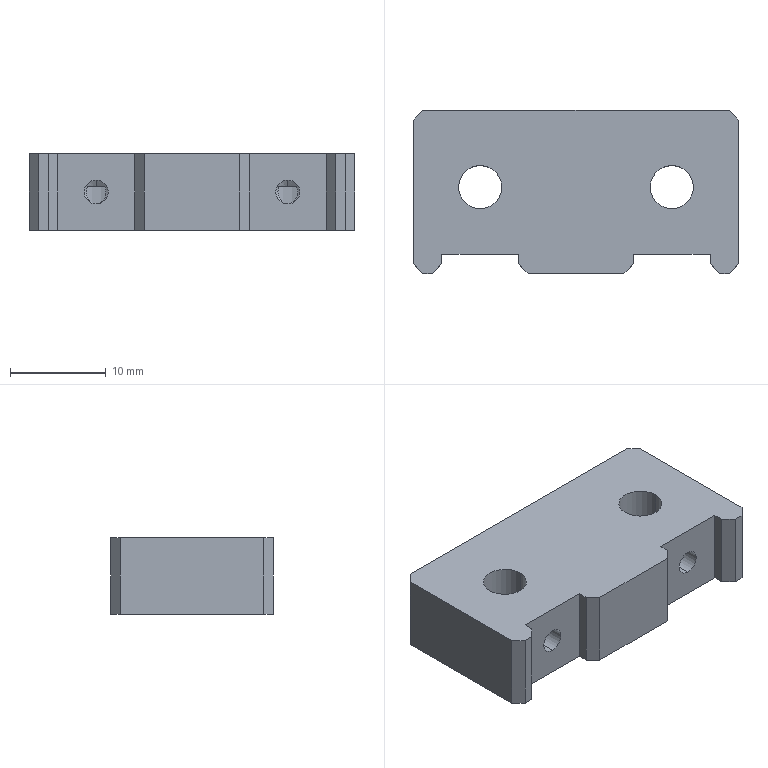Part | SolidWorks | features MirrorStock 1 | 1 solid | 40 faces | box 34 x 17 x 8 mm | volume 3735 mm3 | plane 24 | cylinder 12 | cone 4 | commonest cylinder face diameters 2.5 x4 4.5 x4 8 x4
STEP:
#1=CARTESIAN_POINT('',(10.,-27.5,-2.75));
#2=VERTEX_POINT('',#1);
#3=CARTESIAN_POINT('',(10.,-27.5,-5.25));
#4=VERTEX_POINT('',#3);
#5=CARTESIAN_POINT('',(10.,-27.5,-4.));
#6=DIRECTION('',(0.,1.,0.));
#7=DIRECTION('',(0.,0.,1.));
#8=AXIS2_PLACEMENT_3D('',#5,#6,#7);
#9=CIRCLE('',#8,1.25);
#10=EDGE_CURVE('',#2,#4,#9,.T.);
#11=ORIENTED_EDGE('',*,*,#10,.T.);
#12=CARTESIAN_POINT('',(10.,-30.5,-5.25));
#13=VERTEX_POINT('',#12);
#14=CARTESIAN_POINT('',(10.,-30.5,-5.25));
#15=DIRECTION('',(0.,-1.,0.));
#16=VECTOR('',#15,1000.);
#17=LINE('',#14,#16);
#18=EDGE_CURVE('',#4,#13,#17,.T.);
#19=ORIENTED_EDGE('',*,*,#18,.T.);
#20=CARTESIAN_POINT('',(10.,-30.5,-2.75));
#21=VERTEX_POINT('',#20);
#22=CARTESIAN_POINT('',(10.,-30.5,-4.));
#23=DIRECTION('',(0.,1.,0.));
#24=DIRECTION('',(0.,0.,1.));
#25=AXIS2_PLACEMENT_3D('',#22,#23,#24);
#26=CIRCLE('',#25,1.25);
#27=EDGE_CURVE('',#21,#13,#26,.T.);
#28=ORIENTED_EDGE('',*,*,#27,.F.);
#29=CARTESIAN_POINT('',(10.,-30.5,-2.75));
#30=DIRECTION('',(0.,-1.,0.));
#31=VECTOR('',#30,1000.);
#32=LINE('',#29,#31);
#33=EDGE_CURVE('',#2,#21,#32,.T.);
#34=ORIENTED_EDGE('',*,*,#33,.F.);
#35=EDGE_LOOP('',(#11,#19,#28,#34));
#36=FACE_OUTER_BOUND('',#35,.T.);
#37=CARTESIAN_POINT('',(10.,-30.5,-4.));
#38=DIRECTION('',(0.,-1.,0.));
#39=DIRECTION('',(0.,0.,1.));
#40=AXIS2_PLACEMENT_3D('',#37,#38,#39);
#41=CYLINDRICAL_SURFACE('',#40,1.25);
#42=ADVANCED_FACE('',(#36),#41,.F.);
#43=CARTESIAN_POINT('',(9.102,-27.398,-3.4));
#44=VERTEX_POINT('',#43);
#45=CARTESIAN_POINT('',(10.,-27.109,-3.4));
#46=VERTEX_POINT('',#45);
#47=CARTESIAN_POINT('',(9.102,-27.398,-3.4));
#48=CARTESIAN_POINT('',(9.244,-27.327,-3.4));
#49=CARTESIAN_POINT('',(9.387,-27.259,-3.4));
#50=CARTESIAN_POINT('',(9.686,-27.15,-3.4));
#51=CARTESIAN_POINT('',(9.84,-27.109,-3.4));
#52=CARTESIAN_POINT('',(10.,-27.109,-3.4));
#53=B_SPLINE_CURVE_WITH_KNOTS('',3,(#47,#48,#49,#50,#51,#52),.UNSPECIFIED.,.F.,.F.,(4,2,4),(0.006438,0.006913,0.007389),.UNSPECIFIED.);
#54=EDGE_CURVE('',#44,#46,#53,.T.);
#55=ORIENTED_EDGE('',*,*,#54,.T.);
#56=CARTESIAN_POINT('',(10.,-27.5,-2.75));
#57=DIRECTION('',(0.,-0.515,0.8572));
#58=VECTOR('',#57,1000.);
#59=LINE('',#56,#58);
#60=EDGE_CURVE('',#46,#2,#59,.T.);
#61=ORIENTED_EDGE('',*,*,#60,.T.);
#62=CARTESIAN_POINT('',(10.,-27.5,-4.));
#63=DIRECTION('',(0.,1.,0.));
#64=DIRECTION('',(0.,0.,1.));
#65=AXIS2_PLACEMENT_3D('',#62,#63,#64);
#66=CIRCLE('',#65,1.25);
#67=EDGE_CURVE('',#4,#2,#66,.T.);
#68=ORIENTED_EDGE('',*,*,#67,.F.);
#69=CARTESIAN_POINT('',(10.,-27.5,-5.25));
#70=CARTESIAN_POINT('',(9.9,-27.5,-5.25));
#71=CARTESIAN_POINT('',(9.798,-27.496,-5.231));
#72=CARTESIAN_POINT('',(9.611,-27.482,-5.161));
#73=CARTESIAN_POINT('',(9.522,-27.472,-5.109));
#74=CARTESIAN_POINT('',(9.287,-27.439,-4.922));
#75=CARTESIAN_POINT('',(9.167,-27.413,-4.753));
#76=CARTESIAN_POINT('',(9.01,-27.376,-4.386));
#77=CARTESIAN_POINT('',(8.971,-27.365,-4.184));
#78=CARTESIAN_POINT('',(8.974,-27.366,-3.883));
#79=CARTESIAN_POINT('',(8.986,-27.369,-3.781));
#80=CARTESIAN_POINT('',(9.029,-27.38,-3.586));
#81=CARTESIAN_POINT('',(9.06,-27.388,-3.492));
#82=CARTESIAN_POINT('',(9.102,-27.398,-3.4));
#83=B_SPLINE_CURVE_WITH_KNOTS('',3,(#69,#70,#71,#72,#73,#74,#75,#76,#77,#78,#79,#80,#81,#82),.UNSPECIFIED.,.F.,.F.,(4,2,2,2,2,2,4),(0.002615,0.002915,0.003214,0.003814,0.004413,0.004712,0.005012),.UNSPECIFIED.);
#84=EDGE_CURVE('',#4,#44,#83,.T.);
#85=ORIENTED_EDGE('',*,*,#84,.T.);
#86=EDGE_LOOP('',(#55,#61,#68,#85));
#87=FACE_OUTER_BOUND('',#86,.T.);
#88=CARTESIAN_POINT('',(10.,-27.5,-4.));
#89=DIRECTION('',(0.,-1.,0.));
#90=DIRECTION('',(0.,0.,1.));
#91=AXIS2_PLACEMENT_3D('',#88,#89,#90);
#92=CONICAL_SURFACE('',#91,1.25,1.03);
#93=ADVANCED_FACE('',(#87),#92,.F.);
#94=CARTESIAN_POINT('',(-10.,-27.5,-2.75));
#95=VERTEX_POINT('',#94);
#96=CARTESIAN_POINT('',(-10.,-27.5,-5.25));
#97=VERTEX_POINT('',#96);
#98=CARTESIAN_POINT('',(-10.,-27.5,-4.));
#99=DIRECTION('',(0.,1.,0.));
#100=DIRECTION('',(0.,0.,1.));
#101=AXIS2_PLACEMENT_3D('',#98,#99,#100);
#102=CIRCLE('',#101,1.25);
#103=EDGE_CURVE('',#95,#97,#102,.T.);
#104=ORIENTED_EDGE('',*,*,#103,.T.);
#105=CARTESIAN_POINT('',(-10.,-30.5,-5.25));
#106=VERTEX_POINT('',#105);
#107=CARTESIAN_POINT('',(-10.,-30.5,-5.25));
#108=DIRECTION('',(0.,-1.,0.));
#109=VECTOR('',#108,1000.);
#110=LINE('',#107,#109);
#111=EDGE_CURVE('',#97,#106,#110,.T.);
#112=ORIENTED_EDGE('',*,*,#111,.T.);
#113=CARTESIAN_POINT('',(-10.,-30.5,-2.75));
#114=VERTEX_POINT('',#113);
#115=CARTESIAN_POINT('',(-10.,-30.5,-4.));
#116=DIRECTION('',(0.,1.,0.));
#117=DIRECTION('',(0.,0.,1.));
#118=AXIS2_PLACEMENT_3D('',#115,#116,#117);
#119=CIRCLE('',#118,1.25);
#120=EDGE_CURVE('',#114,#106,#119,.T.);
#121=ORIENTED_EDGE('',*,*,#120,.F.);
#122=CARTESIAN_POINT('',(-10.,-30.5,-2.75));
#123=DIRECTION('',(0.,-1.,0.));
#124=VECTOR('',#123,1000.);
#125=LINE('',#122,#124);
#126=EDGE_CURVE('',#95,#114,#125,.T.);
#127=ORIENTED_EDGE('',*,*,#126,.F.);
#128=EDGE_LOOP('',(#104,#112,#121,#127));
#129=FACE_OUTER_BOUND('',#128,.T.);
#130=CARTESIAN_POINT('',(-10.,-30.5,-4.));
#131=DIRECTION('',(0.,-1.,0.));
#132=DIRECTION('',(0.,0.,1.));
#133=AXIS2_PLACEMENT_3D('',#130,#131,#132);
#134=CYLINDRICAL_SURFACE('',#133,1.25);
#135=ADVANCED_FACE('',(#129),#134,.F.);
#136=CARTESIAN_POINT('',(-10.898,-27.398,-3.4));
#137=VERTEX_POINT('',#136);
#138=CARTESIAN_POINT('',(-10.,-27.109,-3.4));
#139=VERTEX_POINT('',#138);
#140=CARTESIAN_POINT('',(-10.898,-27.398,-3.4));
#141=CARTESIAN_POINT('',(-10.756,-27.327,-3.4));
#142=CARTESIAN_POINT('',(-10.613,-27.259,-3.4));
#143=CARTESIAN_POINT('',(-10.314,-27.15,-3.4));
#144=CARTESIAN_POINT('',(-10.16,-27.109,-3.4));
#145=CARTESIAN_POINT('',(-10.,-27.109,-3.4));
#146=B_SPLINE_CURVE_WITH_KNOTS('',3,(#140,#141,#142,#143,#144,#145),.UNSPECIFIED.,.F.,.F.,(4,2,4),(0.006438,0.006913,0.007389),.UNSPECIFIED.);
#147=EDGE_CURVE('',#137,#139,#146,.T.);
#148=ORIENTED_EDGE('',*,*,#147,.T.);
#149=CARTESIAN_POINT('',(-10.,-27.5,-2.75));
#150=DIRECTION('',(0.,-0.515,0.8572));
#151=VECTOR('',#150,1000.);
#152=LINE('',#149,#151);
#153=EDGE_CURVE('',#139,#95,#152,.T.);
#154=ORIENTED_EDGE('',*,*,#153,.T.);
#155=CARTESIAN_POINT('',(-10.,-27.5,-4.));
#156=DIRECTION('',(0.,1.,0.));
#157=DIRECTION('',(0.,0.,1.));
#158=AXIS2_PLACEMENT_3D('',#155,#156,#157);
#159=CIRCLE('',#158,1.25);
#160=EDGE_CURVE('',#97,#95,#159,.T.);
#161=ORIENTED_EDGE('',*,*,#160,.F.);
#162=CARTESIAN_POINT('',(-10.,-27.5,-5.25));
#163=CARTESIAN_POINT('',(-10.1,-27.5,-5.25));
#164=CARTESIAN_POINT('',(-10.202,-27.496,-5.231));
#165=CARTESIAN_POINT('',(-10.389,-27.482,-5.161));
#166=CARTESIAN_POINT('',(-10.478,-27.472,-5.109));
#167=CARTESIAN_POINT('',(-10.713,-27.439,-4.922));
#168=CARTESIAN_POINT('',(-10.833,-27.413,-4.753));
#169=CARTESIAN_POINT('',(-10.99,-27.376,-4.386));
#170=CARTESIAN_POINT('',(-11.029,-27.365,-4.184));
#171=CARTESIAN_POINT('',(-11.026,-27.366,-3.883));
#172=CARTESIAN_POINT('',(-11.014,-27.369,-3.781));
#173=CARTESIAN_POINT('',(-10.971,-27.38,-3.586));
#174=CARTESIAN_POINT('',(-10.94,-27.388,-3.492));
#175=CARTESIAN_POINT('',(-10.898,-27.398,-3.4));
#176=B_SPLINE_CURVE_WITH_KNOTS('',3,(#162,#163,#164,#165,#166,#167,#168,#169,#170,#171,#172,#173,#174,#175),.UNSPECIFIED.,.F.,.F.,(4,2,2,2,2,2,4),(0.002615,0.002915,0.003214,0.003814,0.004413,0.004712,0.005012),.UNSPECIFIED.);
#177=EDGE_CURVE('',#97,#137,#176,.T.);
#178=ORIENTED_EDGE('',*,*,#177,.T.);
#179=EDGE_LOOP('',(#148,#154,#161,#178));
#180=FACE_OUTER_BOUND('',#179,.T.);
#181=CARTESIAN_POINT('',(-10.,-27.5,-4.));
#182=DIRECTION('',(0.,-1.,0.));
#183=DIRECTION('',(0.,0.,1.));
#184=AXIS2_PLACEMENT_3D('',#181,#182,#183);
#185=CONICAL_SURFACE('',#184,1.25,1.03);
#186=ADVANCED_FACE('',(#180),#185,.F.);
#187=CARTESIAN_POINT('',(14.,-23.5,-3.4));
#188=VERTEX_POINT('',#187);
#189=CARTESIAN_POINT('',(6.,-23.5,-3.4));
#190=VERTEX_POINT('',#189);
#191=CARTESIAN_POINT('',(10.,-23.5,-3.4));
#192=DIRECTION('',(0.,0.,1.));
#193=DIRECTION('',(1.,0.,0.));
#194=AXIS2_PLACEMENT_3D('',#191,#192,#193);
#195=CIRCLE('',#194,4.);
#196=EDGE_CURVE('',#188,#190,#195,.T.);
#197=ORIENTED_EDGE('',*,*,#196,.T.);
#198=CARTESIAN_POINT('',(6.,-23.5,-8.));
#199=VERTEX_POINT('',#198);
#200=CARTESIAN_POINT('',(6.,-23.5,-8.));
#201=DIRECTION('',(0.,0.,-1.));
#202=VECTOR('',#201,1000.);
#203=LINE('',#200,#202);
#204=EDGE_CURVE('',#190,#199,#203,.T.);
#205=ORIENTED_EDGE('',*,*,#204,.T.);
#206=CARTESIAN_POINT('',(14.,-23.5,-8.));
#207=VERTEX_POINT('',#206);
#208=CARTESIAN_POINT('',(10.,-23.5,-8.));
#209=DIRECTION('',(0.,0.,1.));
#210=DIRECTION('',(1.,0.,0.));
#211=AXIS2_PLACEMENT_3D('',#208,#209,#210);
#212=CIRCLE('',#211,4.);
#213=EDGE_CURVE('',#207,#199,#212,.T.);
#214=ORIENTED_EDGE('',*,*,#213,.F.);
#215=CARTESIAN_POINT('',(14.,-23.5,-8.));
#216=DIRECTION('',(0.,0.,-1.));
#217=VECTOR('',#216,1000.);
#218=LINE('',#215,#217);
#219=EDGE_CURVE('',#188,#207,#218,.T.);
#220=ORIENTED_EDGE('',*,*,#219,.F.);
#221=EDGE_LOOP('',(#197,#205,#214,#220));
#222=FACE_OUTER_BOUND('',#221,.T.);
#223=CARTESIAN_POINT('',(10.,-23.5,-8.));
#224=DIRECTION('',(0.,0.,-1.));
#225=DIRECTION('',(1.,0.,0.));
#226=AXIS2_PLACEMENT_3D('',#223,#224,#225);
#227=CYLINDRICAL_SURFACE('',#226,4.);
#228=ADVANCED_FACE('',(#222),#227,.F.);
#229=CARTESIAN_POINT('',(12.25,-23.5,0.));
#230=VERTEX_POINT('',#229);
#231=CARTESIAN_POINT('',(7.75,-23.5,0.));
#232=VERTEX_POINT('',#231);
#233=CARTESIAN_POINT('',(10.,-23.5,0.));
#234=DIRECTION('',(0.,0.,1.));
#235=DIRECTION('',(1.,0.,0.));
#236=AXIS2_PLACEMENT_3D('',#233,#234,#235);
#237=CIRCLE('',#236,2.25);
#238=EDGE_CURVE('',#230,#232,#237,.T.);
#239=ORIENTED_EDGE('',*,*,#238,.T.);
#240=CARTESIAN_POINT('',(7.75,-23.5,-3.4));
#241=VERTEX_POINT('',#240);
#242=CARTESIAN_POINT('',(7.75,-23.5,-8.));
#243=DIRECTION('',(0.,0.,-1.));
#244=VECTOR('',#243,1000.);
#245=LINE('',#242,#244);
#246=EDGE_CURVE('',#232,#241,#245,.T.);
#247=ORIENTED_EDGE('',*,*,#246,.T.);
#248=CARTESIAN_POINT('',(12.25,-23.5,-3.4));
#249=VERTEX_POINT('',#248);
#250=CARTESIAN_POINT('',(10.,-23.5,-3.4));
#251=DIRECTION('',(0.,0.,1.));
#252=DIRECTION('',(1.,0.,0.));
#253=AXIS2_PLACEMENT_3D('',#250,#251,#252);
#254=CIRCLE('',#253,2.25);
#255=EDGE_CURVE('',#249,#241,#254,.T.);
#256=ORIENTED_EDGE('',*,*,#255,.F.);
#257=CARTESIAN_POINT('',(12.25,-23.5,-8.));
#258=DIRECTION('',(0.,0.,-1.));
#259=VECTOR('',#258,1000.);
#260=LINE('',#257,#259);
#261=EDGE_CURVE('',#230,#249,#260,.T.);
#262=ORIENTED_EDGE('',*,*,#261,.F.);
#263=EDGE_LOOP('',(#239,#247,#256,#262));
#264=FACE_OUTER_BOUND('',#263,.T.);
#265=CARTESIAN_POINT('',(10.,-23.5,-8.));
#266=DIRECTION('',(0.,0.,-1.));
#267=DIRECTION('',(1.,0.,0.));
#268=AXIS2_PLACEMENT_3D('',#265,#266,#267);
#269=CYLINDRICAL_SURFACE('',#268,2.25);
#270=ADVANCED_FACE('',(#264),#269,.F.);
#271=CARTESIAN_POINT('',(-6.,-23.5,-3.4));
#272=VERTEX_POINT('',#271);
#273=CARTESIAN_POINT('',(-14.,-23.5,-3.4));
#274=VERTEX_POINT('',#273);
#275=CARTESIAN_POINT('',(-10.,-23.5,-3.4));
#276=DIRECTION('',(0.,0.,1.));
#277=DIRECTION('',(1.,0.,0.));
#278=AXIS2_PLACEMENT_3D('',#275,#276,#277);
#279=CIRCLE('',#278,4.);
#280=EDGE_CURVE('',#272,#274,#279,.T.);
#281=ORIENTED_EDGE('',*,*,#280,.T.);
#282=CARTESIAN_POINT('',(-14.,-23.5,-8.));
#283=VERTEX_POINT('',#282);
#284=CARTESIAN_POINT('',(-14.,-23.5,-8.));
#285=DIRECTION('',(0.,0.,-1.));
#286=VECTOR('',#285,1000.);
#287=LINE('',#284,#286);
#288=EDGE_CURVE('',#274,#283,#287,.T.);
#289=ORIENTED_EDGE('',*,*,#288,.T.);
#290=CARTESIAN_POINT('',(-6.,-23.5,-8.));
#291=VERTEX_POINT('',#290);
#292=CARTESIAN_POINT('',(-10.,-23.5,-8.));
#293=DIRECTION('',(0.,0.,1.));
#294=DIRECTION('',(1.,0.,0.));
#295=AXIS2_PLACEMENT_3D('',#292,#293,#294);
#296=CIRCLE('',#295,4.);
#297=EDGE_CURVE('',#291,#283,#296,.T.);
#298=ORIENTED_EDGE('',*,*,#297,.F.);
#299=CARTESIAN_POINT('',(-6.,-23.5,-8.));
#300=DIRECTION('',(0.,0.,-1.));
#301=VECTOR('',#300,1000.);
#302=LINE('',#299,#301);
#303=EDGE_CURVE('',#272,#291,#302,.T.);
#304=ORIENTED_EDGE('',*,*,#303,.F.);
#305=EDGE_LOOP('',(#281,#289,#298,#304));
#306=FACE_OUTER_BOUND('',#305,.T.);
#307=CARTESIAN_POINT('',(-10.,-23.5,-8.));
#308=DIRECTION('',(0.,0.,-1.));
#309=DIRECTION('',(1.,0.,0.));
#310=AXIS2_PLACEMENT_3D('',#307,#308,#309);
#311=CYLINDRICAL_SURFACE('',#310,4.);
#312=ADVANCED_FACE('',(#306),#311,.F.);
#313=CARTESIAN_POINT('',(-7.75,-23.5,0.));
#314=VERTEX_POINT('',#313);
#315=CARTESIAN_POINT('',(-12.25,-23.5,0.));
#316=VERTEX_POINT('',#315);
#317=CARTESIAN_POINT('',(-10.,-23.5,0.));
#318=DIRECTION('',(0.,0.,1.));
#319=DIRECTION('',(1.,0.,0.));
#320=AXIS2_PLACEMENT_3D('',#317,#318,#319);
#321=CIRCLE('',#320,2.25);
#322=EDGE_CURVE('',#314,#316,#321,.T.);
#323=ORIENTED_EDGE('',*,*,#322,.T.);
#324=CARTESIAN_POINT('',(-12.25,-23.5,-3.4));
#325=VERTEX_POINT('',#324);
#326=CARTESIAN_POINT('',(-12.25,-23.5,-8.));
#327=DIRECTION('',(0.,0.,-1.));
#328=VECTOR('',#327,1000.);
#329=LINE('',#326,#328);
#330=EDGE_CURVE('',#316,#325,#329,.T.);
#331=ORIENTED_EDGE('',*,*,#330,.T.);
#332=CARTESIAN_POINT('',(-7.75,-23.5,-3.4));
#333=VERTEX_POINT('',#332);
#334=CARTESIAN_POINT('',(-10.,-23.5,-3.4));
#335=DIRECTION('',(0.,0.,1.));
#336=DIRECTION('',(1.,0.,0.));
#337=AXIS2_PLACEMENT_3D('',#334,#335,#336);
#338=CIRCLE('',#337,2.25);
#339=EDGE_CURVE('',#333,#325,#338,.T.);
#340=ORIENTED_EDGE('',*,*,#339,.F.);
#341=CARTESIAN_POINT('',(-7.75,-23.5,-8.));
#342=DIRECTION('',(0.,0.,-1.));
#343=VECTOR('',#342,1000.);
#344=LINE('',#341,#343);
#345=EDGE_CURVE('',#314,#333,#344,.T.);
#346=ORIENTED_EDGE('',*,*,#345,.F.);
#347=EDGE_LOOP('',(#323,#331,#340,#346));
#348=FACE_OUTER_BOUND('',#347,.T.);
#349=CARTESIAN_POINT('',(-10.,-23.5,-8.));
#350=DIRECTION('',(0.,0.,-1.));
#351=DIRECTION('',(1.,0.,0.));
#352=AXIS2_PLACEMENT_3D('',#349,#350,#351);
#353=CYLINDRICAL_SURFACE('',#352,2.25);
#354=ADVANCED_FACE('',(#348),#353,.F.);
#355=ORIENTED_EDGE('',*,*,#27,.T.);
#356=CARTESIAN_POINT('',(10.,-30.5,-4.));
#357=DIRECTION('',(0.,1.,0.));
#358=DIRECTION('',(0.,0.,1.));
#359=AXIS2_PLACEMENT_3D('',#356,#357,#358);
#360=CIRCLE('',#359,1.25);
#361=EDGE_CURVE('',#13,#21,#360,.T.);
#362=ORIENTED_EDGE('',*,*,#361,.T.);
#363=EDGE_LOOP('',(#355,#362));
#364=FACE_BOUND('',#363,.T.);
#365=CARTESIAN_POINT('',(6.,-30.5,0.));
#366=VERTEX_POINT('',#365);
#367=CARTESIAN_POINT('',(6.,-30.5,-8.));
#368=VERTEX_POINT('',#367);
#369=CARTESIAN_POINT('',(6.,-30.5,0.));
#370=DIRECTION('',(0.,0.,-1.));
#371=VECTOR('',#370,1000.);
#372=LINE('',#369,#371);
#373=EDGE_CURVE('',#366,#368,#372,.T.);
#374=ORIENTED_EDGE('',*,*,#373,.T.);
#375=CARTESIAN_POINT('',(14.,-30.5,-8.));
#376=VERTEX_POINT('',#375);
#377=CARTESIAN_POINT('',(17.,-30.5,-8.));
#378=DIRECTION('',(-1.,0.,0.));
#379=VECTOR('',#378,1000.);
#380=LINE('',#377,#379);
#381=EDGE_CURVE('',#376,#368,#380,.T.);
#382=ORIENTED_EDGE('',*,*,#381,.F.);
#383=CARTESIAN_POINT('',(14.,-30.5,0.));
#384=VERTEX_POINT('',#383);
#385=CARTESIAN_POINT('',(14.,-30.5,0.));
#386=DIRECTION('',(0.,0.,-1.));
#387=VECTOR('',#386,1000.);
#388=LINE('',#385,#387);
#389=EDGE_CURVE('',#384,#376,#388,.T.);
#390=ORIENTED_EDGE('',*,*,#389,.F.);
#391=CARTESIAN_POINT('',(17.,-30.5,0.));
#392=DIRECTION('',(-1.,0.,0.));
#393=VECTOR('',#392,1000.);
#394=LINE('',#391,#393);
#395=EDGE_CURVE('',#384,#366,#394,.T.);
#396=ORIENTED_EDGE('',*,*,#395,.T.);
#397=EDGE_LOOP('',(#374,#382,#390,#396));
#398=FACE_OUTER_BOUND('',#397,.T.);
#399=CARTESIAN_POINT('',(17.,-30.5,-8.));
#400=DIRECTION('',(0.,-1.,0.));
#401=DIRECTION('',(0.,0.,1.));
#402=AXIS2_PLACEMENT_3D('',#399,#400,#401);
#403=PLANE('',#402);
#404=ADVANCED_FACE('',(#364,#398),#403,.T.);
#405=ORIENTED_EDGE('',*,*,#120,.T.);
#406=CARTESIAN_POINT('',(-10.,-30.5,-4.));
#407=DIRECTION('',(0.,1.,0.));
#408=DIRECTION('',(0.,0.,1.));
#409=AXIS2_PLACEMENT_3D('',#406,#407,#408);
#410=CIRCLE('',#409,1.25);
#411=EDGE_CURVE('',#106,#114,#410,.T.);
#412=ORIENTED_EDGE('',*,*,#411,.T.);
#413=EDGE_LOOP('',(#405,#412));
#414=FACE_BOUND('',#413,.T.);
#415=CARTESIAN_POINT('',(-6.,-30.5,0.));
#416=VERTEX_POINT('',#415);
#417=CARTESIAN_POINT('',(-6.,-30.5,-8.));
#418=VERTEX_POINT('',#417);
#419=CARTESIAN_POINT('',(-6.,-30.5,0.));
#420=DIRECTION('',(0.,0.,-1.));
#421=VECTOR('',#420,1000.);
#422=LINE('',#419,#421);
#423=EDGE_CURVE('',#416,#418,#422,.T.);
#424=ORIENTED_EDGE('',*,*,#423,.F.);
#425=CARTESIAN_POINT('',(-14.,-30.5,0.));
#426=VERTEX_POINT('',#425);
#427=CARTESIAN_POINT('',(17.,-30.5,0.));
#428=DIRECTION('',(-1.,0.,0.));
#429=VECTOR('',#428,1000.);
#430=LINE('',#427,#429);
#431=EDGE_CURVE('',#416,#426,#430,.T.);
#432=ORIENTED_EDGE('',*,*,#431,.T.);
#433=CARTESIAN_POINT('',(-14.,-30.5,-8.));
#434=VERTEX_POINT('',#433);
#435=CARTESIAN_POINT('',(-14.,-30.5,0.));
#436=DIRECTION('',(0.,0.,-1.));
#437=VECTOR('',#436,1000.);
#438=LINE('',#435,#437);
#439=EDGE_CURVE('',#426,#434,#438,.T.);
#440=ORIENTED_EDGE('',*,*,#439,.T.);
#441=CARTESIAN_POINT('',(17.,-30.5,-8.));
#442=DIRECTION('',(-1.,0.,0.));
#443=VECTOR('',#442,1000.);
#444=LINE('',#441,#443);
#445=EDGE_CURVE('',#418,#434,#444,.T.);
#446=ORIENTED_EDGE('',*,*,#445,.F.);
#447=EDGE_LOOP('',(#424,#432,#440,#446));
#448=FACE_OUTER_BOUND('',#447,.T.);
#449=CARTESIAN_POINT('',(17.,-30.5,-8.));
#450=DIRECTION('',(0.,-1.,0.));
#451=DIRECTION('',(0.,0.,1.));
#452=AXIS2_PLACEMENT_3D('',#449,#450,#451);
#453=PLANE('',#452);
#454=ADVANCED_FACE('',(#414,#448),#453,.T.);
#455=CARTESIAN_POINT('',(17.,-31.5,0.));
#456=VERTEX_POINT('',#455);
#457=CARTESIAN_POINT('',(17.,-16.5,0.));
#458=VERTEX_POINT('',#457);
#459=CARTESIAN_POINT('',(17.,-30.5,0.));
#460=DIRECTION('',(0.,1.,0.));
#461=VECTOR('',#460,1000.);
#462=LINE('',#459,#461);
#463=EDGE_CURVE('',#456,#458,#462,.T.);
#464=ORIENTED_EDGE('',*,*,#463,.F.);
#465=CARTESIAN_POINT('',(17.,-31.5,-8.));
#466=VERTEX_POINT('',#465);
#467=CARTESIAN_POINT('',(17.,-31.5,0.));
#468=DIRECTION('',(0.,0.,1.));
#469=VECTOR('',#468,1000.);
#470=LINE('',#467,#469);
#471=EDGE_CURVE('',#466,#456,#470,.T.);
#472=ORIENTED_EDGE('',*,*,#471,.F.);
#473=CARTESIAN_POINT('',(17.,-16.5,-8.));
#474=VERTEX_POINT('',#473);
#475=CARTESIAN_POINT('',(17.,-30.5,-8.));
#476=DIRECTION('',(0.,1.,0.));
#477=VECTOR('',#476,1000.);
#478=LINE('',#475,#477);
#479=EDGE_CURVE('',#466,#474,#478,.T.);
#480=ORIENTED_EDGE('',*,*,#479,.T.);
#481=CARTESIAN_POINT('',(17.,-16.5,-8.));
#482=DIRECTION('',(0.,0.,-1.));
#483=VECTOR('',#482,1000.);
#484=LINE('',#481,#483);
#485=EDGE_CURVE('',#458,#474,#484,.T.);
#486=ORIENTED_EDGE('',*,*,#485,.F.);
#487=EDGE_LOOP('',(#464,#472,#480,#486));
#488=FACE_OUTER_BOUND('',#487,.T.);
#489=CARTESIAN_POINT('',(17.,-30.5,-8.));
#490=DIRECTION('',(-1.,0.,0.));
#491=DIRECTION('',(0.,0.,-1.));
#492=AXIS2_PLACEMENT_3D('',#489,#490,#491);
#493=PLANE('',#492);
#494=ADVANCED_FACE('',(#488),#493,.F.);
#495=CARTESIAN_POINT('',(16.,-15.5,0.));
#496=VERTEX_POINT('',#495);
#497=CARTESIAN_POINT('',(-16.,-15.5,0.));
#498=VERTEX_POINT('',#497);
#499=CARTESIAN_POINT('',(17.,-15.5,0.));
#500=DIRECTION('',(-1.,0.,0.));
#501=VECTOR('',#500,1000.);
#502=LINE('',#499,#501);
#503=EDGE_CURVE('',#496,#498,#502,.T.);
#504=ORIENTED_EDGE('',*,*,#503,.F.);
#505=CARTESIAN_POINT('',(16.,-15.5,-8.));
#506=VERTEX_POINT('',#505);
#507=CARTESIAN_POINT('',(16.,-15.5,-8.));
#508=DIRECTION('',(0.,0.,1.));
#509=VECTOR('',#508,1000.);
#510=LINE('',#507,#509);
#511=EDGE_CURVE('',#506,#496,#510,.T.);
#512=ORIENTED_EDGE('',*,*,#511,.F.);
#513=CARTESIAN_POINT('',(-16.,-15.5,-8.));
#514=VERTEX_POINT('',#513);
#515=CARTESIAN_POINT('',(17.,-15.5,-8.));
#516=DIRECTION('',(-1.,0.,0.));
#517=VECTOR('',#516,1000.);
#518=LINE('',#515,#517);
#519=EDGE_CURVE('',#506,#514,#518,.T.);
#520=ORIENTED_EDGE('',*,*,#519,.T.);
#521=CARTESIAN_POINT('',(-16.,-15.5,-8.));
#522=DIRECTION('',(0.,0.,-1.));
#523=VECTOR('',#522,1000.);
#524=LINE('',#521,#523);
#525=EDGE_CURVE('',#498,#514,#524,.T.);
#526=ORIENTED_EDGE('',*,*,#525,.F.);
#527=EDGE_LOOP('',(#504,#512,#520,#526));
#528=FACE_OUTER_BOUND('',#527,.T.);
#529=CARTESIAN_POINT('',(17.,-15.5,-8.));
#530=DIRECTION('',(0.,-1.,0.));
#531=DIRECTION('',(0.,0.,1.));
#532=AXIS2_PLACEMENT_3D('',#529,#530,#531);
#533=PLANE('',#532);
#534=ADVANCED_FACE('',(#528),#533,.F.);
#535=CARTESIAN_POINT('',(-17.,-31.5,0.));
#536=VERTEX_POINT('',#535);
#537=CARTESIAN_POINT('',(-17.,-16.5,0.));
#538=VERTEX_POINT('',#537);
#539=CARTESIAN_POINT('',(-17.,-30.5,0.));
#540=DIRECTION('',(0.,1.,0.));
#541=VECTOR('',#540,1000.);
#542=LINE('',#539,#541);
#543=EDGE_CURVE('',#536,#538,#542,.T.);
#544=ORIENTED_EDGE('',*,*,#543,.T.);
#545=CARTESIAN_POINT('',(-17.,-16.5,-8.));
#546=VERTEX_POINT('',#545);
#547=CARTESIAN_POINT('',(-17.,-16.5,0.));
#548=DIRECTION('',(0.,0.,1.));
#549=VECTOR('',#548,1000.);
#550=LINE('',#547,#549);
#551=EDGE_CURVE('',#546,#538,#550,.T.);
#552=ORIENTED_EDGE('',*,*,#551,.F.);
#553=CARTESIAN_POINT('',(-17.,-31.5,-8.));
#554=VERTEX_POINT('',#553);
#555=CARTESIAN_POINT('',(-17.,-30.5,-8.));
#556=DIRECTION('',(0.,1.,0.));
#557=VECTOR('',#556,1000.);
#558=LINE('',#555,#557);
#559=EDGE_CURVE('',#554,#546,#558,.T.);
#560=ORIENTED_EDGE('',*,*,#559,.F.);
#561=CARTESIAN_POINT('',(-17.,-31.5,-8.));
#562=DIRECTION('',(0.,0.,-1.));
#563=VECTOR('',#562,1000.);
#564=LINE('',#561,#563);
#565=EDGE_CURVE('',#536,#554,#564,.T.);
#566=ORIENTED_EDGE('',*,*,#565,.F.);
#567=EDGE_LOOP('',(#544,#552,#560,#566));
#568=FACE_OUTER_BOUND('',#567,.T.);
#569=CARTESIAN_POINT('',(-17.,-30.5,-8.));
#570=DIRECTION('',(-1.,0.,0.));
#571=DIRECTION('',(0.,0.,-1.));
#572=AXIS2_PLACEMENT_3D('',#569,#570,#571);
#573=PLANE('',#572);
#574=ADVANCED_FACE('',(#568),#573,.T.);
#575=ORIENTED_EDGE('',*,*,#213,.T.);
#576=CARTESIAN_POINT('',(10.,-23.5,-8.));
#577=DIRECTION('',(0.,0.,1.));
#578=DIRECTION('',(1.,0.,0.));
#579=AXIS2_PLACEMENT_3D('',#576,#577,#578);
#580=CIRCLE('',#579,4.);
#581=EDGE_CURVE('',#199,#207,#580,.T.);
#582=ORIENTED_EDGE('',*,*,#581,.T.);
#583=EDGE_LOOP('',(#575,#582));
#584=FACE_BOUND('',#583,.T.);
#585=ORIENTED_EDGE('',*,*,#297,.T.);
#586=CARTESIAN_POINT('',(-10.,-23.5,-8.));
#587=DIRECTION('',(0.,0.,1.));
#588=DIRECTION('',(1.,0.,0.));
#589=AXIS2_PLACEMENT_3D('',#586,#587,#588);
#590=CIRCLE('',#589,4.);
#591=EDGE_CURVE('',#283,#291,#590,.T.);
#592=ORIENTED_EDGE('',*,*,#591,.T.);
#593=EDGE_LOOP('',(#585,#592));
#594=FACE_BOUND('',#593,.T.);
#595=CARTESIAN_POINT('',(14.,-31.5,-8.));
#596=VERTEX_POINT('',#595);
#597=CARTESIAN_POINT('',(14.,-32.5,-8.));
#598=DIRECTION('',(0.,-1.,0.));
#599=VECTOR('',#598,1000.);
#600=LINE('',#597,#599);
#601=EDGE_CURVE('',#376,#596,#600,.T.);
#602=ORIENTED_EDGE('',*,*,#601,.F.);
#603=ORIENTED_EDGE('',*,*,#381,.T.);
#604=CARTESIAN_POINT('',(6.,-31.5,-8.));
#605=VERTEX_POINT('',#604);
#606=CARTESIAN_POINT('',(6.,-32.5,-8.));
#607=DIRECTION('',(0.,1.,0.));
#608=VECTOR('',#607,1000.);
#609=LINE('',#606,#608);
#610=EDGE_CURVE('',#605,#368,#609,.T.);
#611=ORIENTED_EDGE('',*,*,#610,.F.);
#612=CARTESIAN_POINT('',(5.,-32.5,-8.));
#613=VERTEX_POINT('',#612);
#614=CARTESIAN_POINT('',(18.75,-18.75,-8.));
#615=DIRECTION('',(0.7071,0.7071,0.));
#616=VECTOR('',#615,1000.);
#617=LINE('',#614,#616);
#618=EDGE_CURVE('',#613,#605,#617,.T.);
#619=ORIENTED_EDGE('',*,*,#618,.F.);
#620=CARTESIAN_POINT('',(-5.,-32.5,-8.));
#621=VERTEX_POINT('',#620);
#622=CARTESIAN_POINT('',(6.,-32.5,-8.));
#623=DIRECTION('',(1.,0.,0.));
#624=VECTOR('',#623,1000.);
#625=LINE('',#622,#624);
#626=EDGE_CURVE('',#621,#613,#625,.T.);
#627=ORIENTED_EDGE('',*,*,#626,.F.);
#628=CARTESIAN_POINT('',(-6.,-31.5,-8.));
#629=VERTEX_POINT('',#628);
#630=CARTESIAN_POINT('',(-18.75,-18.75,-8.));
#631=DIRECTION('',(0.7071,-0.7071,0.));
#632=VECTOR('',#631,1000.);
#633=LINE('',#630,#632);
#634=EDGE_CURVE('',#629,#621,#633,.T.);
#635=ORIENTED_EDGE('',*,*,#634,.F.);
#636=CARTESIAN_POINT('',(-6.,-30.5,-8.));
#637=DIRECTION('',(0.,-1.,0.));
#638=VECTOR('',#637,1000.);
#639=LINE('',#636,#638);
#640=EDGE_CURVE('',#418,#629,#639,.T.);
#641=ORIENTED_EDGE('',*,*,#640,.F.);
#642=ORIENTED_EDGE('',*,*,#445,.T.);
#643=CARTESIAN_POINT('',(-14.,-31.5,-8.));
#644=VERTEX_POINT('',#643);
#645=CARTESIAN_POINT('',(-14.,-30.5,-8.));
#646=DIRECTION('',(0.,1.,0.));
#647=VECTOR('',#646,1000.);
#648=LINE('',#645,#647);
#649=EDGE_CURVE('',#644,#434,#648,.T.);
#650=ORIENTED_EDGE('',*,*,#649,.F.);
#651=CARTESIAN_POINT('',(-15.,-32.5,-8.));
#652=VERTEX_POINT('',#651);
#653=CARTESIAN_POINT('',(8.75,-8.75,-8.));
#654=DIRECTION('',(0.7071,0.7071,0.));
#655=VECTOR('',#654,1000.);
#656=LINE('',#653,#655);
#657=EDGE_CURVE('',#652,#644,#656,.T.);
#658=ORIENTED_EDGE('',*,*,#657,.F.);
#659=CARTESIAN_POINT('',(-16.,-32.5,-8.));
#660=VERTEX_POINT('',#659);
#661=CARTESIAN_POINT('',(-14.,-32.5,-8.));
#662=DIRECTION('',(1.,0.,0.));
#663=VECTOR('',#662,1000.);
#664=LINE('',#661,#663);
#665=EDGE_CURVE('',#660,#652,#664,.T.);
#666=ORIENTED_EDGE('',*,*,#665,.F.);
#667=CARTESIAN_POINT('',(-24.25,-24.25,-8.));
#668=DIRECTION('',(0.7071,-0.7071,0.));
#669=VECTOR('',#668,1000.);
#670=LINE('',#667,#669);
#671=EDGE_CURVE('',#554,#660,#670,.T.);
#672=ORIENTED_EDGE('',*,*,#671,.F.);
#673=ORIENTED_EDGE('',*,*,#559,.T.);
#674=CARTESIAN_POINT('',(-0.25,0.25,-8.));
#675=DIRECTION('',(-0.7071,-0.7071,0.));
#676=VECTOR('',#675,1000.);
#677=LINE('',#674,#676);
#678=EDGE_CURVE('',#514,#546,#677,.T.);
#679=ORIENTED_EDGE('',*,*,#678,.F.);
#680=ORIENTED_EDGE('',*,*,#519,.F.);
#681=CARTESIAN_POINT('',(0.25,0.25,-8.));
#682=DIRECTION('',(-0.7071,0.7071,0.));
#683=VECTOR('',#682,1000.);
#684=LINE('',#681,#683);
#685=EDGE_CURVE('',#474,#506,#684,.T.);
#686=ORIENTED_EDGE('',*,*,#685,.F.);
#687=ORIENTED_EDGE('',*,*,#479,.F.);
#688=CARTESIAN_POINT('',(16.,-32.5,-8.));
#689=VERTEX_POINT('',#688);
#690=CARTESIAN_POINT('',(24.25,-24.25,-8.));
#691=DIRECTION('',(0.7071,0.7071,0.));
#692=VECTOR('',#691,1000.);
#693=LINE('',#690,#692);
#694=EDGE_CURVE('',#689,#466,#693,.T.);
#695=ORIENTED_EDGE('',*,*,#694,.F.);
#696=CARTESIAN_POINT('',(15.,-32.5,-8.));
#697=VERTEX_POINT('',#696);
#698=CARTESIAN_POINT('',(17.,-32.5,-8.));
#699=DIRECTION('',(1.,0.,0.));
#700=VECTOR('',#699,1000.);
#701=LINE('',#698,#700);
#702=EDGE_CURVE('',#697,#689,#701,.T.);
#703=ORIENTED_EDGE('',*,*,#702,.F.);
#704=CARTESIAN_POINT('',(-8.75,-8.75,-8.));
#705=DIRECTION('',(0.7071,-0.7071,0.));
#706=VECTOR('',#705,1000.);
#707=LINE('',#704,#706);
#708=EDGE_CURVE('',#596,#697,#707,.T.);
#709=ORIENTED_EDGE('',*,*,#708,.F.);
#710=EDGE_LOOP('',(#602,#603,#611,#619,#627,#635,#641,#642,#650,#658,#666,#672,#673,#679,#680,#686,#687,#695,#703,#709));
#711=FACE_OUTER_BOUND('',#710,.T.);
#712=CARTESIAN_POINT('',(0.,0.,-8.));
#713=DIRECTION('',(0.,0.,-1.));
#714=DIRECTION('',(1.,0.,0.));
#715=AXIS2_PLACEMENT_3D('',#712,#713,#714);
#716=PLANE('',#715);
#717=ADVANCED_FACE('',(#584,#594,#711),#716,.T.);
#718=ORIENTED_EDGE('',*,*,#238,.F.);
#719=CARTESIAN_POINT('',(10.,-23.5,0.));
#720=DIRECTION('',(0.,0.,1.));
#721=DIRECTION('',(1.,0.,0.));
#722=AXIS2_PLACEMENT_3D('',#719,#720,#721);
#723=CIRCLE('',#722,2.25);
#724=EDGE_CURVE('',#232,#230,#723,.T.);
#725=ORIENTED_EDGE('',*,*,#724,.F.);
#726=EDGE_LOOP('',(#718,#725));
#727=FACE_BOUND('',#726,.T.);
#728=ORIENTED_EDGE('',*,*,#322,.F.);
#729=CARTESIAN_POINT('',(-10.,-23.5,0.));
#730=DIRECTION('',(0.,0.,1.));
#731=DIRECTION('',(1.,0.,0.));
#732=AXIS2_PLACEMENT_3D('',#729,#730,#731);
#733=CIRCLE('',#732,2.25);
#734=EDGE_CURVE('',#316,#314,#733,.T.);
#735=ORIENTED_EDGE('',*,*,#734,.F.);
#736=EDGE_LOOP('',(#728,#735));
#737=FACE_BOUND('',#736,.T.);
#738=CARTESIAN_POINT('',(15.,-32.5,0.));
#739=VERTEX_POINT('',#738);
#740=CARTESIAN_POINT('',(16.,-32.5,0.));
#741=VERTEX_POINT('',#740);
#742=CARTESIAN_POINT('',(17.,-32.5,0.));
#743=DIRECTION('',(1.,0.,0.));
#744=VECTOR('',#743,1000.);
#745=LINE('',#742,#744);
#746=EDGE_CURVE('',#739,#741,#745,.T.);
#747=ORIENTED_EDGE('',*,*,#746,.T.);
#748=CARTESIAN_POINT('',(16.,-32.5,0.));
#749=DIRECTION('',(-0.7071,-0.7071,0.));
#750=VECTOR('',#749,1000.);
#751=LINE('',#748,#750);
#752=EDGE_CURVE('',#456,#741,#751,.T.);
#753=ORIENTED_EDGE('',*,*,#752,.F.);
#754=ORIENTED_EDGE('',*,*,#463,.T.);
#755=CARTESIAN_POINT('',(16.,-15.5,0.));
#756=DIRECTION('',(0.7071,-0.7071,0.));
#757=VECTOR('',#756,1000.);
#758=LINE('',#755,#757);
#759=EDGE_CURVE('',#496,#458,#758,.T.);
#760=ORIENTED_EDGE('',*,*,#759,.F.);
#761=ORIENTED_EDGE('',*,*,#503,.T.);
#762=CARTESIAN_POINT('',(-17.,-16.5,0.));
#763=DIRECTION('',(0.7071,0.7071,0.));
#764=VECTOR('',#763,1000.);
#765=LINE('',#762,#764);
#766=EDGE_CURVE('',#538,#498,#765,.T.);
#767=ORIENTED_EDGE('',*,*,#766,.F.);
#768=ORIENTED_EDGE('',*,*,#543,.F.);
#769=CARTESIAN_POINT('',(-16.,-32.5,0.));
#770=VERTEX_POINT('',#769);
#771=CARTESIAN_POINT('',(-17.,-31.5,0.));
#772=DIRECTION('',(-0.7071,0.7071,0.));
#773=VECTOR('',#772,1000.);
#774=LINE('',#771,#773);
#775=EDGE_CURVE('',#770,#536,#774,.T.);
#776=ORIENTED_EDGE('',*,*,#775,.F.);
#777=CARTESIAN_POINT('',(-15.,-32.5,0.));
#778=VERTEX_POINT('',#777);
#779=CARTESIAN_POINT('',(-14.,-32.5,0.));
#780=DIRECTION('',(1.,0.,0.));
#781=VECTOR('',#780,1000.);
#782=LINE('',#779,#781);
#783=EDGE_CURVE('',#770,#778,#782,.T.);
#784=ORIENTED_EDGE('',*,*,#783,.T.);
#785=CARTESIAN_POINT('',(-14.,-31.5,0.));
#786=VERTEX_POINT('',#785);
#787=CARTESIAN_POINT('',(-15.,-32.5,0.));
#788=DIRECTION('',(-0.7071,-0.7071,0.));
#789=VECTOR('',#788,1000.);
#790=LINE('',#787,#789);
#791=EDGE_CURVE('',#786,#778,#790,.T.);
#792=ORIENTED_EDGE('',*,*,#791,.F.);
#793=CARTESIAN_POINT('',(-14.,-30.5,0.));
#794=DIRECTION('',(0.,1.,0.));
#795=VECTOR('',#794,1000.);
#796=LINE('',#793,#795);
#797=EDGE_CURVE('',#786,#426,#796,.T.);
#798=ORIENTED_EDGE('',*,*,#797,.T.);
#799=ORIENTED_EDGE('',*,*,#431,.F.);
#800=CARTESIAN_POINT('',(-6.,-31.5,0.));
#801=VERTEX_POINT('',#800);
#802=CARTESIAN_POINT('',(-6.,-30.5,0.));
#803=DIRECTION('',(0.,-1.,0.));
#804=VECTOR('',#803,1000.);
#805=LINE('',#802,#804);
#806=EDGE_CURVE('',#416,#801,#805,.T.);
#807=ORIENTED_EDGE('',*,*,#806,.T.);
#808=CARTESIAN_POINT('',(-5.,-32.5,0.));
#809=VERTEX_POINT('',#808);
#810=CARTESIAN_POINT('',(-6.,-31.5,0.));
#811=DIRECTION('',(-0.7071,0.7071,0.));
#812=VECTOR('',#811,1000.);
#813=LINE('',#810,#812);
#814=EDGE_CURVE('',#809,#801,#813,.T.);
#815=ORIENTED_EDGE('',*,*,#814,.F.);
#816=CARTESIAN_POINT('',(5.,-32.5,0.));
#817=VERTEX_POINT('',#816);
#818=CARTESIAN_POINT('',(6.,-32.5,0.));
#819=DIRECTION('',(1.,0.,0.));
#820=VECTOR('',#819,1000.);
#821=LINE('',#818,#820);
#822=EDGE_CURVE('',#809,#817,#821,.T.);
#823=ORIENTED_EDGE('',*,*,#822,.T.);
#824=CARTESIAN_POINT('',(6.,-31.5,0.));
#825=VERTEX_POINT('',#824);
#826=CARTESIAN_POINT('',(5.,-32.5,0.));
#827=DIRECTION('',(-0.7071,-0.7071,0.));
#828=VECTOR('',#827,1000.);
#829=LINE('',#826,#828);
#830=EDGE_CURVE('',#825,#817,#829,.T.);
#831=ORIENTED_EDGE('',*,*,#830,.F.);
#832=CARTESIAN_POINT('',(6.,-32.5,0.));
#833=DIRECTION('',(0.,1.,0.));
#834=VECTOR('',#833,1000.);
#835=LINE('',#832,#834);
#836=EDGE_CURVE('',#825,#366,#835,.T.);
#837=ORIENTED_EDGE('',*,*,#836,.T.);
#838=ORIENTED_EDGE('',*,*,#395,.F.);
#839=CARTESIAN_POINT('',(14.,-31.5,0.));
#840=VERTEX_POINT('',#839);
#841=CARTESIAN_POINT('',(14.,-32.5,0.));
#842=DIRECTION('',(0.,-1.,0.));
#843=VECTOR('',#842,1000.);
#844=LINE('',#841,#843);
#845=EDGE_CURVE('',#384,#840,#844,.T.);
#846=ORIENTED_EDGE('',*,*,#845,.T.);
#847=CARTESIAN_POINT('',(14.,-31.5,0.));
#848=DIRECTION('',(-0.7071,0.7071,0.));
#849=VECTOR('',#848,1000.);
#850=LINE('',#847,#849);
#851=EDGE_CURVE('',#739,#840,#850,.T.);
#852=ORIENTED_EDGE('',*,*,#851,.F.);
#853=EDGE_LOOP('',(#747,#753,#754,#760,#761,#767,#768,#776,#784,#792,#798,#799,#807,#815,#823,#831,#837,#838,#846,#852));
#854=FACE_OUTER_BOUND('',#853,.T.);
#855=CARTESIAN_POINT('',(0.,0.,0.));
#856=DIRECTION('',(0.,0.,-1.));
#857=DIRECTION('',(1.,0.,0.));
#858=AXIS2_PLACEMENT_3D('',#855,#856,#857);
#859=PLANE('',#858);
#860=ADVANCED_FACE('',(#727,#737,#854),#859,.F.);
#861=ORIENTED_EDGE('',*,*,#702,.T.);
#862=CARTESIAN_POINT('',(16.,-32.5,-8.));
#863=DIRECTION('',(0.,0.,-1.));
#864=VECTOR('',#863,1000.);
#865=LINE('',#862,#864);
#866=EDGE_CURVE('',#741,#689,#865,.T.);
#867=ORIENTED_EDGE('',*,*,#866,.F.);
#868=ORIENTED_EDGE('',*,*,#746,.F.);
#869=CARTESIAN_POINT('',(15.,-32.5,0.));
#870=DIRECTION('',(0.,0.,1.));
#871=VECTOR('',#870,1000.);
#872=LINE('',#869,#871);
#873=EDGE_CURVE('',#697,#739,#872,.T.);
#874=ORIENTED_EDGE('',*,*,#873,.F.);
#875=EDGE_LOOP('',(#861,#867,#868,#874));
#876=FACE_OUTER_BOUND('',#875,.T.);
#877=CARTESIAN_POINT('',(17.,-32.5,0.));
#878=DIRECTION('',(0.,-1.,0.));
#879=DIRECTION('',(0.,0.,1.));
#880=AXIS2_PLACEMENT_3D('',#877,#878,#879);
#881=PLANE('',#880);
#882=ADVANCED_FACE('',(#876),#881,.T.);
#883=ORIENTED_EDGE('',*,*,#845,.F.);
#884=ORIENTED_EDGE('',*,*,#389,.T.);
#885=ORIENTED_EDGE('',*,*,#601,.T.);
#886=CARTESIAN_POINT('',(14.,-31.5,0.));
#887=DIRECTION('',(0.,0.,-1.));
#888=VECTOR('',#887,1000.);
#889=LINE('',#886,#888);
#890=EDGE_CURVE('',#840,#596,#889,.T.);
#891=ORIENTED_EDGE('',*,*,#890,.F.);
#892=EDGE_LOOP('',(#883,#884,#885,#891));
#893=FACE_OUTER_BOUND('',#892,.T.);
#894=CARTESIAN_POINT('',(14.,-32.5,0.));
#895=DIRECTION('',(-1.,0.,0.));
#896=DIRECTION('',(0.,-1.,0.));
#897=AXIS2_PLACEMENT_3D('',#894,#895,#896);
#898=PLANE('',#897);
#899=ADVANCED_FACE('',(#893),#898,.T.);
#900=ORIENTED_EDGE('',*,*,#783,.F.);
#901=CARTESIAN_POINT('',(-16.,-32.5,0.));
#902=DIRECTION('',(0.,0.,1.));
#903=VECTOR('',#902,1000.);
#904=LINE('',#901,#903);
#905=EDGE_CURVE('',#660,#770,#904,.T.);
#906=ORIENTED_EDGE('',*,*,#905,.F.);
#907=ORIENTED_EDGE('',*,*,#665,.T.);
#908=CARTESIAN_POINT('',(-15.,-32.5,0.));
#909=DIRECTION('',(0.,0.,-1.));
#910=VECTOR('',#909,1000.);
#911=LINE('',#908,#910);
#912=EDGE_CURVE('',#778,#652,#911,.T.);
#913=ORIENTED_EDGE('',*,*,#912,.F.);
#914=EDGE_LOOP('',(#900,#906,#907,#913));
#915=FACE_OUTER_BOUND('',#914,.T.);
#916=CARTESIAN_POINT('',(-14.,-32.5,0.));
#917=DIRECTION('',(0.,-1.,0.));
#918=DIRECTION('',(0.,0.,1.));
#919=AXIS2_PLACEMENT_3D('',#916,#917,#918);
#920=PLANE('',#919);
#921=ADVANCED_FACE('',(#915),#920,.T.);
#922=ORIENTED_EDGE('',*,*,#649,.T.);
#923=ORIENTED_EDGE('',*,*,#439,.F.);
#924=ORIENTED_EDGE('',*,*,#797,.F.);
#925=CARTESIAN_POINT('',(-14.,-31.5,0.));
#926=DIRECTION('',(0.,0.,1.));
#927=VECTOR('',#926,1000.);
#928=LINE('',#925,#927);
#929=EDGE_CURVE('',#644,#786,#928,.T.);
#930=ORIENTED_EDGE('',*,*,#929,.F.);
#931=EDGE_LOOP('',(#922,#923,#924,#930));
#932=FACE_OUTER_BOUND('',#931,.T.);
#933=CARTESIAN_POINT('',(-14.,-30.5,0.));
#934=DIRECTION('',(1.,0.,0.));
#935=DIRECTION('',(0.,0.,1.));
#936=AXIS2_PLACEMENT_3D('',#933,#934,#935);
#937=PLANE('',#936);
#938=ADVANCED_FACE('',(#932),#937,.T.);
#939=ORIENTED_EDGE('',*,*,#610,.T.);
#940=ORIENTED_EDGE('',*,*,#373,.F.);
#941=ORIENTED_EDGE('',*,*,#836,.F.);
#942=CARTESIAN_POINT('',(6.,-31.5,0.));
#943=DIRECTION('',(0.,0.,1.));
#944=VECTOR('',#943,1000.);
#945=LINE('',#942,#944);
#946=EDGE_CURVE('',#605,#825,#945,.T.);
#947=ORIENTED_EDGE('',*,*,#946,.F.);
#948=EDGE_LOOP('',(#939,#940,#941,#947));
#949=FACE_OUTER_BOUND('',#948,.T.);
#950=CARTESIAN_POINT('',(6.,-32.5,0.));
#951=DIRECTION('',(1.,0.,0.));
#952=DIRECTION('',(0.,1.,0.));
#953=AXIS2_PLACEMENT_3D('',#950,#951,#952);
#954=PLANE('',#953);
#955=ADVANCED_FACE('',(#949),#954,.T.);
#956=ORIENTED_EDGE('',*,*,#626,.T.);
#957=CARTESIAN_POINT('',(5.,-32.5,0.));
#958=DIRECTION('',(0.,0.,-1.));
#959=VECTOR('',#958,1000.);
#960=LINE('',#957,#959);
#961=EDGE_CURVE('',#817,#613,#960,.T.);
#962=ORIENTED_EDGE('',*,*,#961,.F.);
#963=ORIENTED_EDGE('',*,*,#822,.F.);
#964=CARTESIAN_POINT('',(-5.,-32.5,0.));
#965=DIRECTION('',(0.,0.,1.));
#966=VECTOR('',#965,1000.);
#967=LINE('',#964,#966);
#968=EDGE_CURVE('',#621,#809,#967,.T.);
#969=ORIENTED_EDGE('',*,*,#968,.F.);
#970=EDGE_LOOP('',(#956,#962,#963,#969));
#971=FACE_OUTER_BOUND('',#970,.T.);
#972=CARTESIAN_POINT('',(6.,-32.5,0.));
#973=DIRECTION('',(0.,-1.,0.));
#974=DIRECTION('',(1.,0.,0.));
#975=AXIS2_PLACEMENT_3D('',#972,#973,#974);
#976=PLANE('',#975);
#977=ADVANCED_FACE('',(#971),#976,.T.);
#978=ORIENTED_EDGE('',*,*,#806,.F.);
#979=ORIENTED_EDGE('',*,*,#423,.T.);
#980=ORIENTED_EDGE('',*,*,#640,.T.);
#981=CARTESIAN_POINT('',(-6.,-31.5,0.));
#982=DIRECTION('',(0.,0.,-1.));
#983=VECTOR('',#982,1000.);
#984=LINE('',#981,#983);
#985=EDGE_CURVE('',#801,#629,#984,.T.);
#986=ORIENTED_EDGE('',*,*,#985,.F.);
#987=EDGE_LOOP('',(#978,#979,#980,#986));
#988=FACE_OUTER_BOUND('',#987,.T.);
#989=CARTESIAN_POINT('',(-6.,-30.5,0.));
#990=DIRECTION('',(-1.,0.,0.));
#991=DIRECTION('',(0.,0.,-1.));
#992=AXIS2_PLACEMENT_3D('',#989,#990,#991);
#993=PLANE('',#992);
#994=ADVANCED_FACE('',(#988),#993,.T.);
#995=ORIENTED_EDGE('',*,*,#330,.F.);
#996=ORIENTED_EDGE('',*,*,#734,.T.);
#997=ORIENTED_EDGE('',*,*,#345,.T.);
#998=CARTESIAN_POINT('',(-10.,-23.5,-3.4));
#999=DIRECTION('',(0.,0.,1.));
#1000=DIRECTION('',(1.,0.,0.));
#1001=AXIS2_PLACEMENT_3D('',#998,#999,#1000);
#1002=CIRCLE('',#1001,2.25);
#1003=EDGE_CURVE('',#325,#333,#1002,.T.);
#1004=ORIENTED_EDGE('',*,*,#1003,.F.);
#1005=EDGE_LOOP('',(#995,#996,#997,#1004));
#1006=FACE_OUTER_BOUND('',#1005,.T.);
#1007=CARTESIAN_POINT('',(-10.,-23.5,-8.));
#1008=DIRECTION('',(0.,0.,-1.));
#1009=DIRECTION('',(1.,0.,0.));
#1010=AXIS2_PLACEMENT_3D('',#1007,#1008,#1009);
#1011=CYLINDRICAL_SURFACE('',#1010,2.25);
#1012=ADVANCED_FACE('',(#1006),#1011,.F.);
#1013=ORIENTED_EDGE('',*,*,#339,.T.);
#1014=ORIENTED_EDGE('',*,*,#1003,.T.);
#1015=EDGE_LOOP('',(#1013,#1014));
#1016=FACE_BOUND('',#1015,.T.);
#1017=CARTESIAN_POINT('',(-9.102,-27.398,-3.4));
#1018=VERTEX_POINT('',#1017);
#1019=CARTESIAN_POINT('',(-10.,-23.5,-3.4));
#1020=DIRECTION('',(0.,0.,1.));
#1021=DIRECTION('',(1.,0.,0.));
#1022=AXIS2_PLACEMENT_3D('',#1019,#1020,#1021);
#1023=CIRCLE('',#1022,4.);
#1024=EDGE_CURVE('',#1018,#272,#1023,.T.);
#1025=ORIENTED_EDGE('',*,*,#1024,.F.);
#1026=CARTESIAN_POINT('',(-10.,-27.109,-3.4));
#1027=CARTESIAN_POINT('',(-9.84,-27.109,-3.4));
#1028=CARTESIAN_POINT('',(-9.685,-27.15,-3.4));
#1029=CARTESIAN_POINT('',(-9.386,-27.26,-3.4));
#1030=CARTESIAN_POINT('',(-9.243,-27.327,-3.4));
#1031=CARTESIAN_POINT('',(-9.102,-27.398,-3.4));
#1032=B_SPLINE_CURVE_WITH_KNOTS('',3,(#1026,#1027,#1028,#1029,#1030,#1031),.UNSPECIFIED.,.F.,.F.,(4,2,4),(0.007389,0.007867,0.008344),.UNSPECIFIED.);
#1033=EDGE_CURVE('',#139,#1018,#1032,.T.);
#1034=ORIENTED_EDGE('',*,*,#1033,.F.);
#1035=ORIENTED_EDGE('',*,*,#147,.F.);
#1036=CARTESIAN_POINT('',(-10.,-23.5,-3.4));
#1037=DIRECTION('',(0.,0.,1.));
#1038=DIRECTION('',(1.,0.,0.));
#1039=AXIS2_PLACEMENT_3D('',#1036,#1037,#1038);
#1040=CIRCLE('',#1039,4.);
#1041=EDGE_CURVE('',#274,#137,#1040,.T.);
#1042=ORIENTED_EDGE('',*,*,#1041,.F.);
#1043=ORIENTED_EDGE('',*,*,#280,.F.);
#1044=EDGE_LOOP('',(#1025,#1034,#1035,#1042,#1043));
#1045=FACE_OUTER_BOUND('',#1044,.T.);
#1046=CARTESIAN_POINT('',(-7.75,-23.5,-3.4));
#1047=DIRECTION('',(0.,0.,1.));
#1048=DIRECTION('',(-1.,0.,0.));
#1049=AXIS2_PLACEMENT_3D('',#1046,#1047,#1048);
#1050=PLANE('',#1049);
#1051=ADVANCED_FACE('',(#1016,#1045),#1050,.F.);
#1052=ORIENTED_EDGE('',*,*,#288,.F.);
#1053=ORIENTED_EDGE('',*,*,#1041,.T.);
#1054=ORIENTED_EDGE('',*,*,#177,.F.);
#1055=CARTESIAN_POINT('',(-9.102,-27.398,-3.4));
#1056=CARTESIAN_POINT('',(-9.019,-27.379,-3.581));
#1057=CARTESIAN_POINT('',(-8.975,-27.367,-3.782));
#1058=CARTESIAN_POINT('',(-8.971,-27.365,-4.185));
#1059=CARTESIAN_POINT('',(-9.01,-27.376,-4.386));
#1060=CARTESIAN_POINT('',(-9.129,-27.404,-4.663));
#1061=CARTESIAN_POINT('',(-9.178,-27.415,-4.75));
#1062=CARTESIAN_POINT('',(-9.295,-27.438,-4.91));
#1063=CARTESIAN_POINT('',(-9.365,-27.45,-4.984));
#1064=CARTESIAN_POINT('',(-9.521,-27.472,-5.109));
#1065=CARTESIAN_POINT('',(-9.61,-27.482,-5.16));
#1066=CARTESIAN_POINT('',(-9.798,-27.496,-5.231));
#1067=CARTESIAN_POINT('',(-9.9,-27.5,-5.25));
#1068=CARTESIAN_POINT('',(-10.,-27.5,-5.25));
#1069=B_SPLINE_CURVE_WITH_KNOTS('',3,(#1055,#1056,#1057,#1058,#1059,#1060,#1061,#1062,#1063,#1064,#1065,#1066,#1067,#1068),.UNSPECIFIED.,.F.,.F.,(4,2,2,2,2,2,4),(0.0002124,0.0008131,0.001414,0.001714,0.002014,0.002315,0.002615),.UNSPECIFIED.);
#1070=EDGE_CURVE('',#1018,#97,#1069,.T.);
#1071=ORIENTED_EDGE('',*,*,#1070,.F.);
#1072=ORIENTED_EDGE('',*,*,#1024,.T.);
#1073=ORIENTED_EDGE('',*,*,#303,.T.);
#1074=ORIENTED_EDGE('',*,*,#591,.F.);
#1075=EDGE_LOOP('',(#1052,#1053,#1054,#1071,#1072,#1073,#1074));
#1076=FACE_OUTER_BOUND('',#1075,.T.);
#1077=CARTESIAN_POINT('',(-10.,-23.5,-8.));
#1078=DIRECTION('',(0.,0.,-1.));
#1079=DIRECTION('',(1.,0.,0.));
#1080=AXIS2_PLACEMENT_3D('',#1077,#1078,#1079);
#1081=CYLINDRICAL_SURFACE('',#1080,4.);
#1082=ADVANCED_FACE('',(#1076),#1081,.F.);
#1083=ORIENTED_EDGE('',*,*,#246,.F.);
#1084=ORIENTED_EDGE('',*,*,#724,.T.);
#1085=ORIENTED_EDGE('',*,*,#261,.T.);
#1086=CARTESIAN_POINT('',(10.,-23.5,-3.4));
#1087=DIRECTION('',(0.,0.,1.));
#1088=DIRECTION('',(1.,0.,0.));
#1089=AXIS2_PLACEMENT_3D('',#1086,#1087,#1088);
#1090=CIRCLE('',#1089,2.25);
#1091=EDGE_CURVE('',#241,#249,#1090,.T.);
#1092=ORIENTED_EDGE('',*,*,#1091,.F.);
#1093=EDGE_LOOP('',(#1083,#1084,#1085,#1092));
#1094=FACE_OUTER_BOUND('',#1093,.T.);
#1095=CARTESIAN_POINT('',(10.,-23.5,-8.));
#1096=DIRECTION('',(0.,0.,-1.));
#1097=DIRECTION('',(1.,0.,0.));
#1098=AXIS2_PLACEMENT_3D('',#1095,#1096,#1097);
#1099=CYLINDRICAL_SURFACE('',#1098,2.25);
#1100=ADVANCED_FACE('',(#1094),#1099,.F.);
#1101=ORIENTED_EDGE('',*,*,#255,.T.);
#1102=ORIENTED_EDGE('',*,*,#1091,.T.);
#1103=EDGE_LOOP('',(#1101,#1102));
#1104=FACE_BOUND('',#1103,.T.);
#1105=CARTESIAN_POINT('',(10.898,-27.398,-3.4));
#1106=VERTEX_POINT('',#1105);
#1107=CARTESIAN_POINT('',(10.,-23.5,-3.4));
#1108=DIRECTION('',(0.,0.,1.));
#1109=DIRECTION('',(1.,0.,0.));
#1110=AXIS2_PLACEMENT_3D('',#1107,#1108,#1109);
#1111=CIRCLE('',#1110,4.);
#1112=EDGE_CURVE('',#1106,#188,#1111,.T.);
#1113=ORIENTED_EDGE('',*,*,#1112,.F.);
#1114=CARTESIAN_POINT('',(10.,-27.109,-3.4));
#1115=CARTESIAN_POINT('',(10.16,-27.109,-3.4));
#1116=CARTESIAN_POINT('',(10.315,-27.15,-3.4));
#1117=CARTESIAN_POINT('',(10.614,-27.26,-3.4));
#1118=CARTESIAN_POINT('',(10.757,-27.327,-3.4));
#1119=CARTESIAN_POINT('',(10.898,-27.398,-3.4));
#1120=B_SPLINE_CURVE_WITH_KNOTS('',3,(#1114,#1115,#1116,#1117,#1118,#1119),.UNSPECIFIED.,.F.,.F.,(4,2,4),(0.007389,0.007867,0.008344),.UNSPECIFIED.);
#1121=EDGE_CURVE('',#46,#1106,#1120,.T.);
#1122=ORIENTED_EDGE('',*,*,#1121,.F.);
#1123=ORIENTED_EDGE('',*,*,#54,.F.);
#1124=CARTESIAN_POINT('',(10.,-23.5,-3.4));
#1125=DIRECTION('',(0.,0.,1.));
#1126=DIRECTION('',(1.,0.,0.));
#1127=AXIS2_PLACEMENT_3D('',#1124,#1125,#1126);
#1128=CIRCLE('',#1127,4.);
#1129=EDGE_CURVE('',#190,#44,#1128,.T.);
#1130=ORIENTED_EDGE('',*,*,#1129,.F.);
#1131=ORIENTED_EDGE('',*,*,#196,.F.);
#1132=EDGE_LOOP('',(#1113,#1122,#1123,#1130,#1131));
#1133=FACE_OUTER_BOUND('',#1132,.T.);
#1134=CARTESIAN_POINT('',(12.25,-23.5,-3.4));
#1135=DIRECTION('',(0.,0.,1.));
#1136=DIRECTION('',(-1.,0.,0.));
#1137=AXIS2_PLACEMENT_3D('',#1134,#1135,#1136);
#1138=PLANE('',#1137);
#1139=ADVANCED_FACE('',(#1104,#1133),#1138,.F.);
#1140=ORIENTED_EDGE('',*,*,#204,.F.);
#1141=ORIENTED_EDGE('',*,*,#1129,.T.);
#1142=ORIENTED_EDGE('',*,*,#84,.F.);
#1143=CARTESIAN_POINT('',(10.898,-27.398,-3.4));
#1144=CARTESIAN_POINT('',(10.981,-27.379,-3.581));
#1145=CARTESIAN_POINT('',(11.025,-27.367,-3.782));
#1146=CARTESIAN_POINT('',(11.029,-27.365,-4.185));
#1147=CARTESIAN_POINT('',(10.99,-27.376,-4.386));
#1148=CARTESIAN_POINT('',(10.871,-27.404,-4.663));
#1149=CARTESIAN_POINT('',(10.822,-27.415,-4.75));
#1150=CARTESIAN_POINT('',(10.705,-27.438,-4.91));
#1151=CARTESIAN_POINT('',(10.635,-27.45,-4.984));
#1152=CARTESIAN_POINT('',(10.479,-27.472,-5.109));
#1153=CARTESIAN_POINT('',(10.39,-27.482,-5.16));
#1154=CARTESIAN_POINT('',(10.202,-27.496,-5.231));
#1155=CARTESIAN_POINT('',(10.1,-27.5,-5.25));
#1156=CARTESIAN_POINT('',(10.,-27.5,-5.25));
#1157=B_SPLINE_CURVE_WITH_KNOTS('',3,(#1143,#1144,#1145,#1146,#1147,#1148,#1149,#1150,#1151,#1152,#1153,#1154,#1155,#1156),.UNSPECIFIED.,.F.,.F.,(4,2,2,2,2,2,4),(0.0002124,0.0008131,0.001414,0.001714,0.002014,0.002315,0.002615),.UNSPECIFIED.);
#1158=EDGE_CURVE('',#1106,#4,#1157,.T.);
#1159=ORIENTED_EDGE('',*,*,#1158,.F.);
#1160=ORIENTED_EDGE('',*,*,#1112,.T.);
#1161=ORIENTED_EDGE('',*,*,#219,.T.);
#1162=ORIENTED_EDGE('',*,*,#581,.F.);
#1163=EDGE_LOOP('',(#1140,#1141,#1142,#1159,#1160,#1161,#1162));
#1164=FACE_OUTER_BOUND('',#1163,.T.);
#1165=CARTESIAN_POINT('',(10.,-23.5,-8.));
#1166=DIRECTION('',(0.,0.,-1.));
#1167=DIRECTION('',(1.,0.,0.));
#1168=AXIS2_PLACEMENT_3D('',#1165,#1166,#1167);
#1169=CYLINDRICAL_SURFACE('',#1168,4.);
#1170=ADVANCED_FACE('',(#1164),#1169,.F.);
#1171=ORIENTED_EDGE('',*,*,#153,.F.);
#1172=ORIENTED_EDGE('',*,*,#1033,.T.);
#1173=ORIENTED_EDGE('',*,*,#1070,.T.);
#1174=ORIENTED_EDGE('',*,*,#103,.F.);
#1175=EDGE_LOOP('',(#1171,#1172,#1173,#1174));
#1176=FACE_OUTER_BOUND('',#1175,.T.);
#1177=CARTESIAN_POINT('',(-10.,-27.5,-4.));
#1178=DIRECTION('',(0.,-1.,0.));
#1179=DIRECTION('',(0.,0.,1.));
#1180=AXIS2_PLACEMENT_3D('',#1177,#1178,#1179);
#1181=CONICAL_SURFACE('',#1180,1.25,1.03);
#1182=ADVANCED_FACE('',(#1176),#1181,.F.);
#1183=ORIENTED_EDGE('',*,*,#111,.F.);
#1184=ORIENTED_EDGE('',*,*,#160,.T.);
#1185=ORIENTED_EDGE('',*,*,#126,.T.);
#1186=ORIENTED_EDGE('',*,*,#411,.F.);
#1187=EDGE_LOOP('',(#1183,#1184,#1185,#1186));
#1188=FACE_OUTER_BOUND('',#1187,.T.);
#1189=CARTESIAN_POINT('',(-10.,-30.5,-4.));
#1190=DIRECTION('',(0.,-1.,0.));
#1191=DIRECTION('',(0.,0.,1.));
#1192=AXIS2_PLACEMENT_3D('',#1189,#1190,#1191);
#1193=CYLINDRICAL_SURFACE('',#1192,1.25);
#1194=ADVANCED_FACE('',(#1188),#1193,.F.);
#1195=ORIENTED_EDGE('',*,*,#60,.F.);
#1196=ORIENTED_EDGE('',*,*,#1121,.T.);
#1197=ORIENTED_EDGE('',*,*,#1158,.T.);
#1198=ORIENTED_EDGE('',*,*,#10,.F.);
#1199=EDGE_LOOP('',(#1195,#1196,#1197,#1198));
#1200=FACE_OUTER_BOUND('',#1199,.T.);
#1201=CARTESIAN_POINT('',(10.,-27.5,-4.));
#1202=DIRECTION('',(0.,-1.,0.));
#1203=DIRECTION('',(0.,0.,1.));
#1204=AXIS2_PLACEMENT_3D('',#1201,#1202,#1203);
#1205=CONICAL_SURFACE('',#1204,1.25,1.03);
#1206=ADVANCED_FACE('',(#1200),#1205,.F.);
#1207=ORIENTED_EDGE('',*,*,#18,.F.);
#1208=ORIENTED_EDGE('',*,*,#67,.T.);
#1209=ORIENTED_EDGE('',*,*,#33,.T.);
#1210=ORIENTED_EDGE('',*,*,#361,.F.);
#1211=EDGE_LOOP('',(#1207,#1208,#1209,#1210));
#1212=FACE_OUTER_BOUND('',#1211,.T.);
#1213=CARTESIAN_POINT('',(10.,-30.5,-4.));
#1214=DIRECTION('',(0.,-1.,0.));
#1215=DIRECTION('',(0.,0.,1.));
#1216=AXIS2_PLACEMENT_3D('',#1213,#1214,#1215);
#1217=CYLINDRICAL_SURFACE('',#1216,1.25);
#1218=ADVANCED_FACE('',(#1212),#1217,.F.);
#1219=ORIENTED_EDGE('',*,*,#851,.T.);
#1220=ORIENTED_EDGE('',*,*,#890,.T.);
#1221=ORIENTED_EDGE('',*,*,#708,.T.);
#1222=ORIENTED_EDGE('',*,*,#873,.T.);
#1223=EDGE_LOOP('',(#1219,#1220,#1221,#1222));
#1224=FACE_OUTER_BOUND('',#1223,.T.);
#1225=CARTESIAN_POINT('',(14.,-31.5,0.));
#1226=DIRECTION('',(0.7071,0.7071,0.));
#1227=DIRECTION('',(0.,0.,-1.));
#1228=AXIS2_PLACEMENT_3D('',#1225,#1226,#1227);
#1229=PLANE('',#1228);
#1230=ADVANCED_FACE('',(#1224),#1229,.F.);
#1231=ORIENTED_EDGE('',*,*,#791,.T.);
#1232=ORIENTED_EDGE('',*,*,#912,.T.);
#1233=ORIENTED_EDGE('',*,*,#657,.T.);
#1234=ORIENTED_EDGE('',*,*,#929,.T.);
#1235=EDGE_LOOP('',(#1231,#1232,#1233,#1234));
#1236=FACE_OUTER_BOUND('',#1235,.T.);
#1237=CARTESIAN_POINT('',(-15.,-32.5,0.));
#1238=DIRECTION('',(-0.7071,0.7071,0.));
#1239=DIRECTION('',(0.,0.,-1.));
#1240=AXIS2_PLACEMENT_3D('',#1237,#1238,#1239);
#1241=PLANE('',#1240);
#1242=ADVANCED_FACE('',(#1236),#1241,.F.);
#1243=ORIENTED_EDGE('',*,*,#814,.T.);
#1244=ORIENTED_EDGE('',*,*,#985,.T.);
#1245=ORIENTED_EDGE('',*,*,#634,.T.);
#1246=ORIENTED_EDGE('',*,*,#968,.T.);
#1247=EDGE_LOOP('',(#1243,#1244,#1245,#1246));
#1248=FACE_OUTER_BOUND('',#1247,.T.);
#1249=CARTESIAN_POINT('',(-6.,-31.5,0.));
#1250=DIRECTION('',(0.7071,0.7071,0.));
#1251=DIRECTION('',(0.,0.,-1.));
#1252=AXIS2_PLACEMENT_3D('',#1249,#1250,#1251);
#1253=PLANE('',#1252);
#1254=ADVANCED_FACE('',(#1248),#1253,.F.);
#1255=ORIENTED_EDGE('',*,*,#830,.T.);
#1256=ORIENTED_EDGE('',*,*,#961,.T.);
#1257=ORIENTED_EDGE('',*,*,#618,.T.);
#1258=ORIENTED_EDGE('',*,*,#946,.T.);
#1259=EDGE_LOOP('',(#1255,#1256,#1257,#1258));
#1260=FACE_OUTER_BOUND('',#1259,.T.);
#1261=CARTESIAN_POINT('',(5.,-32.5,0.));
#1262=DIRECTION('',(-0.7071,0.7071,0.));
#1263=DIRECTION('',(0.,0.,-1.));
#1264=AXIS2_PLACEMENT_3D('',#1261,#1262,#1263);
#1265=PLANE('',#1264);
#1266=ADVANCED_FACE('',(#1260),#1265,.F.);
#1267=ORIENTED_EDGE('',*,*,#775,.T.);
#1268=ORIENTED_EDGE('',*,*,#565,.T.);
#1269=ORIENTED_EDGE('',*,*,#671,.T.);
#1270=ORIENTED_EDGE('',*,*,#905,.T.);
#1271=EDGE_LOOP('',(#1267,#1268,#1269,#1270));
#1272=FACE_OUTER_BOUND('',#1271,.T.);
#1273=CARTESIAN_POINT('',(-17.,-31.5,-8.));
#1274=DIRECTION('',(0.7071,0.7071,0.));
#1275=DIRECTION('',(0.,0.,-1.));
#1276=AXIS2_PLACEMENT_3D('',#1273,#1274,#1275);
#1277=PLANE('',#1276);
#1278=ADVANCED_FACE('',(#1272),#1277,.F.);
#1279=ORIENTED_EDGE('',*,*,#678,.T.);
#1280=ORIENTED_EDGE('',*,*,#551,.T.);
#1281=ORIENTED_EDGE('',*,*,#766,.T.);
#1282=ORIENTED_EDGE('',*,*,#525,.T.);
#1283=EDGE_LOOP('',(#1279,#1280,#1281,#1282));
#1284=FACE_OUTER_BOUND('',#1283,.T.);
#1285=CARTESIAN_POINT('',(-17.,-16.5,-8.));
#1286=DIRECTION('',(-0.7071,0.7071,0.));
#1287=DIRECTION('',(0.,0.,-1.));
#1288=AXIS2_PLACEMENT_3D('',#1285,#1286,#1287);
#1289=PLANE('',#1288);
#1290=ADVANCED_FACE('',(#1284),#1289,.T.);
#1291=ORIENTED_EDGE('',*,*,#685,.T.);
#1292=ORIENTED_EDGE('',*,*,#511,.T.);
#1293=ORIENTED_EDGE('',*,*,#759,.T.);
#1294=ORIENTED_EDGE('',*,*,#485,.T.);
#1295=EDGE_LOOP('',(#1291,#1292,#1293,#1294));
#1296=FACE_OUTER_BOUND('',#1295,.T.);
#1297=CARTESIAN_POINT('',(16.,-15.5,-8.));
#1298=DIRECTION('',(-0.7071,-0.7071,0.));
#1299=DIRECTION('',(0.,0.,1.));
#1300=AXIS2_PLACEMENT_3D('',#1297,#1298,#1299);
#1301=PLANE('',#1300);
#1302=ADVANCED_FACE('',(#1296),#1301,.F.);
#1303=ORIENTED_EDGE('',*,*,#752,.T.);
#1304=ORIENTED_EDGE('',*,*,#866,.T.);
#1305=ORIENTED_EDGE('',*,*,#694,.T.);
#1306=ORIENTED_EDGE('',*,*,#471,.T.);
#1307=EDGE_LOOP('',(#1303,#1304,#1305,#1306));
#1308=FACE_OUTER_BOUND('',#1307,.T.);
#1309=CARTESIAN_POINT('',(16.,-32.5,0.));
#1310=DIRECTION('',(0.7071,-0.7071,0.));
#1311=DIRECTION('',(0.,0.,1.));
#1312=AXIS2_PLACEMENT_3D('',#1309,#1310,#1311);
#1313=PLANE('',#1312);
#1314=ADVANCED_FACE('',(#1308),#1313,.T.);
#1315=CLOSED_SHELL('',(#42,#93,#135,#186,#228,#270,#312,#354,#404,#454,#494,#534,#574,#717,#860,#882,#899,#921,#938,#955,#977,#994,#1012,#1051,#1082,#1100,#1139,#1170,#1182,#1194,#1206,#1218,#1230,#1242,#1254,#1266,#1278,#1290,#1302,#1314));
#1316=MANIFOLD_SOLID_BREP('',#1315);
#1317=CARTESIAN_POINT('',(0.,0.,0.));
#1318=DIRECTION('',(0.,0.,1.));
#1319=DIRECTION('',(1.,0.,0.));
#1320=AXIS2_PLACEMENT_3D('',#1317,#1318,#1319);
#1321=(LENGTH_UNIT()NAMED_UNIT(*)SI_UNIT(.MILLI.,.METRE.));
#1322=UNCERTAINTY_MEASURE_WITH_UNIT(LENGTH_MEASURE(0.00001),#1321,'','');
#1323=(NAMED_UNIT(*)PLANE_ANGLE_UNIT()SI_UNIT($,.RADIAN.));
#1324=(NAMED_UNIT(*)SI_UNIT($,.STERADIAN.)SOLID_ANGLE_UNIT());
#1325=(GEOMETRIC_REPRESENTATION_CONTEXT(3)GLOBAL_UNCERTAINTY_ASSIGNED_CONTEXT((#1322))GLOBAL_UNIT_ASSIGNED_CONTEXT((#1321,#1323,#1324))REPRESENTATION_CONTEXT('',''));
#1326=ADVANCED_BREP_SHAPE_REPRESENTATION('',(#1316,#1320),#1325);